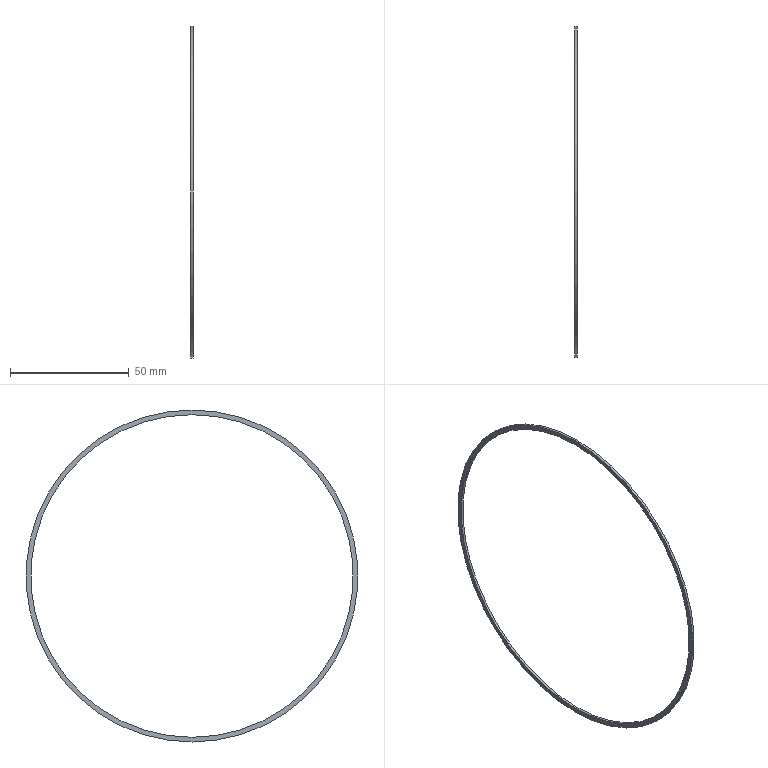Part | STEP file | Outer sealing ring | 1 solid | 4 faces | box 1 x 140 x 140 mm | volume 867.08 mm3 | plane 2 | cylinder 2 | commonest cylinder face diameters 136 x1 140 x1
STEP:
#1=CARTESIAN_POINT('',(0.,0.,-70.));
#2=VERTEX_POINT('',#1);
#3=CARTESIAN_POINT('',(0.,0.,0.));
#4=DIRECTION('',(1.,0.,0.));
#5=DIRECTION('',(0.,0.,-1.));
#6=AXIS2_PLACEMENT_3D('',#3,#4,#5);
#7=CIRCLE('',#6,70.);
#8=EDGE_CURVE('',#2,#2,#7,.T.);
#9=ORIENTED_EDGE('',*,*,#8,.F.);
#10=EDGE_LOOP('',(#9));
#11=FACE_BOUND('',#10,.T.);
#12=CARTESIAN_POINT('',(0.,0.,-68.));
#13=VERTEX_POINT('',#12);
#14=CARTESIAN_POINT('',(0.,0.,0.));
#15=DIRECTION('',(1.,0.,0.));
#16=DIRECTION('',(0.,0.,-1.));
#17=AXIS2_PLACEMENT_3D('',#14,#15,#16);
#18=CIRCLE('',#17,68.);
#19=EDGE_CURVE('',#13,#13,#18,.T.);
#20=ORIENTED_EDGE('',*,*,#19,.T.);
#21=EDGE_LOOP('',(#20));
#22=FACE_BOUND('',#21,.T.);
#23=CARTESIAN_POINT('',(0.,0.,0.));
#24=DIRECTION('',(1.,0.,0.));
#25=DIRECTION('',(0.,0.,-1.));
#26=AXIS2_PLACEMENT_3D('',#23,#24,#25);
#27=PLANE('',#26);
#28=ADVANCED_FACE('',(#11,#22),#27,.F.);
#29=CARTESIAN_POINT('',(1.,0.,-70.));
#30=VERTEX_POINT('',#29);
#31=CARTESIAN_POINT('',(1.,0.,0.));
#32=DIRECTION('',(1.,0.,0.));
#33=DIRECTION('',(0.,0.,-1.));
#34=AXIS2_PLACEMENT_3D('',#31,#32,#33);
#35=CIRCLE('',#34,70.);
#36=EDGE_CURVE('',#30,#30,#35,.T.);
#37=ORIENTED_EDGE('',*,*,#36,.T.);
#38=EDGE_LOOP('',(#37));
#39=FACE_BOUND('',#38,.T.);
#40=CARTESIAN_POINT('',(1.,0.,-68.));
#41=VERTEX_POINT('',#40);
#42=CARTESIAN_POINT('',(1.,0.,0.));
#43=DIRECTION('',(1.,0.,0.));
#44=DIRECTION('',(0.,0.,-1.));
#45=AXIS2_PLACEMENT_3D('',#42,#43,#44);
#46=CIRCLE('',#45,68.);
#47=EDGE_CURVE('',#41,#41,#46,.F.);
#48=ORIENTED_EDGE('',*,*,#47,.T.);
#49=EDGE_LOOP('',(#48));
#50=FACE_BOUND('',#49,.T.);
#51=CARTESIAN_POINT('',(1.,0.,0.));
#52=DIRECTION('',(1.,0.,0.));
#53=DIRECTION('',(0.,0.,-1.));
#54=AXIS2_PLACEMENT_3D('',#51,#52,#53);
#55=PLANE('',#54);
#56=ADVANCED_FACE('',(#39,#50),#55,.T.);
#57=ORIENTED_EDGE('',*,*,#47,.F.);
#58=EDGE_LOOP('',(#57));
#59=FACE_OUTER_BOUND('',#58,.T.);
#60=ORIENTED_EDGE('',*,*,#19,.F.);
#61=EDGE_LOOP('',(#60));
#62=FACE_OUTER_BOUND('',#61,.T.);
#63=CARTESIAN_POINT('',(0.,0.,0.));
#64=DIRECTION('',(1.,0.,0.));
#65=DIRECTION('',(0.,0.,-1.));
#66=AXIS2_PLACEMENT_3D('',#63,#64,#65);
#67=CYLINDRICAL_SURFACE('',#66,68.);
#68=ADVANCED_FACE('',(#59,#62),#67,.F.);
#69=ORIENTED_EDGE('',*,*,#36,.F.);
#70=EDGE_LOOP('',(#69));
#71=FACE_OUTER_BOUND('',#70,.T.);
#72=ORIENTED_EDGE('',*,*,#8,.T.);
#73=EDGE_LOOP('',(#72));
#74=FACE_OUTER_BOUND('',#73,.T.);
#75=CARTESIAN_POINT('',(0.,0.,0.));
#76=DIRECTION('',(1.,0.,0.));
#77=DIRECTION('',(0.,0.,-1.));
#78=AXIS2_PLACEMENT_3D('',#75,#76,#77);
#79=CYLINDRICAL_SURFACE('',#78,70.);
#80=ADVANCED_FACE('',(#71,#74),#79,.T.);
#81=CLOSED_SHELL('',(#28,#56,#68,#80));
#82=MANIFOLD_SOLID_BREP('',#81);
#83=(LENGTH_UNIT()NAMED_UNIT(*)SI_UNIT(.MILLI.,.METRE.));
#84=UNCERTAINTY_MEASURE_WITH_UNIT(LENGTH_MEASURE(0.00001),#83,'','');
#85=(NAMED_UNIT(*)PLANE_ANGLE_UNIT()SI_UNIT($,.RADIAN.));
#86=(NAMED_UNIT(*)SI_UNIT($,.STERADIAN.)SOLID_ANGLE_UNIT());
#87=(GEOMETRIC_REPRESENTATION_CONTEXT(3)GLOBAL_UNCERTAINTY_ASSIGNED_CONTEXT((#84))GLOBAL_UNIT_ASSIGNED_CONTEXT((#83,#85,#86))REPRESENTATION_CONTEXT('',''));
#88=ADVANCED_BREP_SHAPE_REPRESENTATION('',(#82),#87);